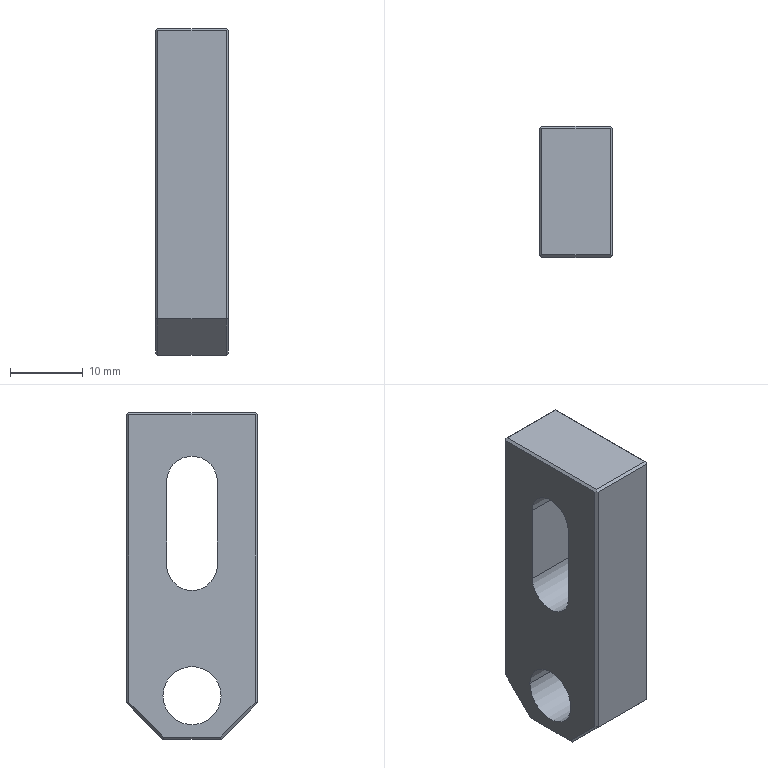Part | NX | 1 solid | 28 faces | box 10 x 18 x 45 mm | volume 6146 mm3 | plane 24 | cylinder 4 | commonest cylinder face diameters 7 x2 8 x2
STEP:
#1=CARTESIAN_POINT('',(-203.3,43.05,26.5));
#2=VERTEX_POINT('',#1);
#3=CARTESIAN_POINT('',(-212.7,43.05,26.5));
#4=VERTEX_POINT('',#3);
#5=CARTESIAN_POINT('',(-208.,43.05,26.5));
#6=DIRECTION('',(-1.,0.,0.));
#7=VECTOR('',#6,1000.);
#8=LINE('',#5,#7);
#9=EDGE_CURVE('',#2,#4,#8,.T.);
#10=ORIENTED_EDGE('',*,*,#9,.F.);
#11=CARTESIAN_POINT('',(-203.3,60.45,26.5));
#12=VERTEX_POINT('',#11);
#13=CARTESIAN_POINT('',(-203.3,51.75,26.5));
#14=DIRECTION('',(0.,1.,0.));
#15=VECTOR('',#14,1000.);
#16=LINE('',#13,#15);
#17=EDGE_CURVE('',#2,#12,#16,.T.);
#18=ORIENTED_EDGE('',*,*,#17,.T.);
#19=CARTESIAN_POINT('',(-212.7,60.45,26.5));
#20=VERTEX_POINT('',#19);
#21=CARTESIAN_POINT('',(-208.,60.45,26.5));
#22=DIRECTION('',(1.,0.,0.));
#23=VECTOR('',#22,1000.);
#24=LINE('',#21,#23);
#25=EDGE_CURVE('',#20,#12,#24,.T.);
#26=ORIENTED_EDGE('',*,*,#25,.F.);
#27=CARTESIAN_POINT('',(-212.7,51.75,26.5));
#28=DIRECTION('',(0.,1.,0.));
#29=VECTOR('',#28,1000.);
#30=LINE('',#27,#29);
#31=EDGE_CURVE('',#4,#20,#30,.T.);
#32=ORIENTED_EDGE('',*,*,#31,.F.);
#33=EDGE_LOOP('',(#10,#18,#26,#32));
#34=FACE_BOUND('',#33,.T.);
#35=CARTESIAN_POINT('',(-203.,60.75,26.5));
#36=DIRECTION('',(0.,0.,1.));
#37=DIRECTION('',(1.,0.,0.));
#38=AXIS2_PLACEMENT_3D('',#35,#36,#37);
#39=PLANE('',#38);
#40=ADVANCED_FACE('',(#34),#39,.T.);
#41=CARTESIAN_POINT('',(-203.3,60.75,-13.5));
#42=VERTEX_POINT('',#41);
#43=CARTESIAN_POINT('',(-212.7,60.75,-13.5));
#44=VERTEX_POINT('',#43);
#45=CARTESIAN_POINT('',(-208.,60.75,-13.5));
#46=DIRECTION('',(-1.,0.,0.));
#47=VECTOR('',#46,1000.);
#48=LINE('',#45,#47);
#49=EDGE_CURVE('',#42,#44,#48,.T.);
#50=ORIENTED_EDGE('',*,*,#49,.T.);
#51=CARTESIAN_POINT('',(-212.7,60.75,26.2));
#52=VERTEX_POINT('',#51);
#53=CARTESIAN_POINT('',(-212.7,60.75,6.5));
#54=DIRECTION('',(0.,0.,-1.));
#55=VECTOR('',#54,1000.);
#56=LINE('',#53,#55);
#57=EDGE_CURVE('',#52,#44,#56,.T.);
#58=ORIENTED_EDGE('',*,*,#57,.F.);
#59=CARTESIAN_POINT('',(-203.3,60.75,26.2));
#60=VERTEX_POINT('',#59);
#61=CARTESIAN_POINT('',(-208.,60.75,26.2));
#62=DIRECTION('',(1.,0.,0.));
#63=VECTOR('',#62,1000.);
#64=LINE('',#61,#63);
#65=EDGE_CURVE('',#52,#60,#64,.T.);
#66=ORIENTED_EDGE('',*,*,#65,.T.);
#67=CARTESIAN_POINT('',(-203.3,60.75,6.5));
#68=DIRECTION('',(0.,0.,-1.));
#69=VECTOR('',#68,1000.);
#70=LINE('',#67,#69);
#71=EDGE_CURVE('',#60,#42,#70,.T.);
#72=ORIENTED_EDGE('',*,*,#71,.T.);
#73=EDGE_LOOP('',(#50,#58,#66,#72));
#74=FACE_BOUND('',#73,.T.);
#75=CARTESIAN_POINT('',(-203.,60.75,0.5));
#76=DIRECTION('',(0.,1.,0.));
#77=DIRECTION('',(1.,0.,0.));
#78=AXIS2_PLACEMENT_3D('',#75,#76,#77);
#79=PLANE('',#78);
#80=ADVANCED_FACE('',(#74),#79,.T.);
#81=CARTESIAN_POINT('',(-212.7,47.75,-18.5));
#82=VERTEX_POINT('',#81);
#83=CARTESIAN_POINT('',(-203.3,47.75,-18.5));
#84=VERTEX_POINT('',#83);
#85=CARTESIAN_POINT('',(-208.,47.75,-18.5));
#86=DIRECTION('',(1.,0.,0.));
#87=VECTOR('',#86,1000.);
#88=LINE('',#85,#87);
#89=EDGE_CURVE('',#82,#84,#88,.T.);
#90=ORIENTED_EDGE('',*,*,#89,.F.);
#91=CARTESIAN_POINT('',(-212.7,55.75,-18.5));
#92=VERTEX_POINT('',#91);
#93=CARTESIAN_POINT('',(-212.7,51.75,-18.5));
#94=DIRECTION('',(0.,-1.,0.));
#95=VECTOR('',#94,1000.);
#96=LINE('',#93,#95);
#97=EDGE_CURVE('',#92,#82,#96,.T.);
#98=ORIENTED_EDGE('',*,*,#97,.F.);
#99=CARTESIAN_POINT('',(-203.3,55.75,-18.5));
#100=VERTEX_POINT('',#99);
#101=CARTESIAN_POINT('',(-208.,55.75,-18.5));
#102=DIRECTION('',(-1.,0.,0.));
#103=VECTOR('',#102,1000.);
#104=LINE('',#101,#103);
#105=EDGE_CURVE('',#100,#92,#104,.T.);
#106=ORIENTED_EDGE('',*,*,#105,.F.);
#107=CARTESIAN_POINT('',(-203.3,51.75,-18.5));
#108=DIRECTION('',(0.,-1.,0.));
#109=VECTOR('',#108,1000.);
#110=LINE('',#107,#109);
#111=EDGE_CURVE('',#100,#84,#110,.T.);
#112=ORIENTED_EDGE('',*,*,#111,.T.);
#113=EDGE_LOOP('',(#90,#98,#106,#112));
#114=FACE_BOUND('',#113,.T.);
#115=CARTESIAN_POINT('',(-203.,42.75,-18.5));
#116=DIRECTION('',(0.,0.,-1.));
#117=DIRECTION('',(0.,-1.,0.));
#118=AXIS2_PLACEMENT_3D('',#115,#116,#117);
#119=PLANE('',#118);
#120=ADVANCED_FACE('',(#114),#119,.T.);
#121=CARTESIAN_POINT('',(-203.3,42.75,-13.5));
#122=VERTEX_POINT('',#121);
#123=CARTESIAN_POINT('',(-203.3,42.75,26.2));
#124=VERTEX_POINT('',#123);
#125=CARTESIAN_POINT('',(-203.3,42.75,6.5));
#126=DIRECTION('',(0.,0.,1.));
#127=VECTOR('',#126,1000.);
#128=LINE('',#125,#127);
#129=EDGE_CURVE('',#122,#124,#128,.T.);
#130=ORIENTED_EDGE('',*,*,#129,.T.);
#131=CARTESIAN_POINT('',(-212.7,42.75,26.2));
#132=VERTEX_POINT('',#131);
#133=CARTESIAN_POINT('',(-208.,42.75,26.2));
#134=DIRECTION('',(-1.,0.,0.));
#135=VECTOR('',#134,1000.);
#136=LINE('',#133,#135);
#137=EDGE_CURVE('',#124,#132,#136,.T.);
#138=ORIENTED_EDGE('',*,*,#137,.T.);
#139=CARTESIAN_POINT('',(-212.7,42.75,-13.5));
#140=VERTEX_POINT('',#139);
#141=CARTESIAN_POINT('',(-212.7,42.75,6.5));
#142=DIRECTION('',(0.,0.,1.));
#143=VECTOR('',#142,1000.);
#144=LINE('',#141,#143);
#145=EDGE_CURVE('',#140,#132,#144,.T.);
#146=ORIENTED_EDGE('',*,*,#145,.F.);
#147=CARTESIAN_POINT('',(-208.,42.75,-13.5));
#148=DIRECTION('',(1.,0.,0.));
#149=VECTOR('',#148,1000.);
#150=LINE('',#147,#149);
#151=EDGE_CURVE('',#140,#122,#150,.T.);
#152=ORIENTED_EDGE('',*,*,#151,.T.);
#153=EDGE_LOOP('',(#130,#138,#146,#152));
#154=FACE_BOUND('',#153,.T.);
#155=CARTESIAN_POINT('',(-203.,42.75,18.5));
#156=DIRECTION('',(0.,-1.,0.));
#157=DIRECTION('',(0.,0.,-1.));
#158=AXIS2_PLACEMENT_3D('',#155,#156,#157);
#159=PLANE('',#158);
#160=ADVANCED_FACE('',(#154),#159,.T.);
#161=CARTESIAN_POINT('',(-203.,55.75,-12.5));
#162=VERTEX_POINT('',#161);
#163=CARTESIAN_POINT('',(-203.,47.75,-12.5));
#164=VERTEX_POINT('',#163);
#165=CARTESIAN_POINT('',(-203.,51.75,-12.5));
#166=DIRECTION('',(-1.,0.,0.));
#167=DIRECTION('',(0.,-1.,0.));
#168=AXIS2_PLACEMENT_3D('',#165,#166,#167);
#169=CIRCLE('',#168,4.);
#170=EDGE_CURVE('',#162,#164,#169,.T.);
#171=ORIENTED_EDGE('',*,*,#170,.F.);
#172=CARTESIAN_POINT('',(-213.,55.75,-12.5));
#173=VERTEX_POINT('',#172);
#174=CARTESIAN_POINT('',(-202.,55.75,-12.5));
#175=DIRECTION('',(-1.,0.,0.));
#176=VECTOR('',#175,1000.);
#177=LINE('',#174,#176);
#178=EDGE_CURVE('',#173,#162,#177,.F.);
#179=ORIENTED_EDGE('',*,*,#178,.F.);
#180=CARTESIAN_POINT('',(-213.,47.75,-12.5));
#181=VERTEX_POINT('',#180);
#182=CARTESIAN_POINT('',(-213.,51.75,-12.5));
#183=DIRECTION('',(-1.,0.,0.));
#184=DIRECTION('',(0.,-1.,0.));
#185=AXIS2_PLACEMENT_3D('',#182,#183,#184);
#186=CIRCLE('',#185,4.);
#187=EDGE_CURVE('',#173,#181,#186,.T.);
#188=ORIENTED_EDGE('',*,*,#187,.T.);
#189=CARTESIAN_POINT('',(-202.,47.75,-12.5));
#190=DIRECTION('',(-1.,0.,0.));
#191=VECTOR('',#190,1000.);
#192=LINE('',#189,#191);
#193=EDGE_CURVE('',#181,#164,#192,.F.);
#194=ORIENTED_EDGE('',*,*,#193,.T.);
#195=EDGE_LOOP('',(#171,#179,#188,#194));
#196=FACE_BOUND('',#195,.T.);
#197=CARTESIAN_POINT('',(-202.,51.75,-12.5));
#198=DIRECTION('',(-1.,0.,0.));
#199=DIRECTION('',(0.,-1.,0.));
#200=AXIS2_PLACEMENT_3D('',#197,#198,#199);
#201=CYLINDRICAL_SURFACE('',#200,4.);
#202=ADVANCED_FACE('',(#196),#201,.F.);
#203=CARTESIAN_POINT('',(-203.3,58.25,-16.));
#204=DIRECTION('',(0.,0.7071,0.7071));
#205=VECTOR('',#204,1000.);
#206=LINE('',#203,#205);
#207=EDGE_CURVE('',#100,#42,#206,.T.);
#208=ORIENTED_EDGE('',*,*,#207,.F.);
#209=ORIENTED_EDGE('',*,*,#105,.T.);
#210=CARTESIAN_POINT('',(-212.7,58.25,-16.));
#211=DIRECTION('',(0.,0.7071,0.7071));
#212=VECTOR('',#211,1000.);
#213=LINE('',#210,#212);
#214=EDGE_CURVE('',#92,#44,#213,.T.);
#215=ORIENTED_EDGE('',*,*,#214,.T.);
#216=ORIENTED_EDGE('',*,*,#49,.F.);
#217=EDGE_LOOP('',(#208,#209,#215,#216));
#218=FACE_BOUND('',#217,.T.);
#219=CARTESIAN_POINT('',(-208.,58.25,-16.));
#220=DIRECTION('',(0.,0.7071,-0.7071));
#221=DIRECTION('',(-1.,0.,0.));
#222=AXIS2_PLACEMENT_3D('',#219,#220,#221);
#223=PLANE('',#222);
#224=ADVANCED_FACE('',(#218),#223,.T.);
#225=CARTESIAN_POINT('',(-203.3,45.25,-16.));
#226=DIRECTION('',(0.,-0.7071,0.7071));
#227=VECTOR('',#226,1000.);
#228=LINE('',#225,#227);
#229=EDGE_CURVE('',#84,#122,#228,.T.);
#230=ORIENTED_EDGE('',*,*,#229,.T.);
#231=ORIENTED_EDGE('',*,*,#151,.F.);
#232=CARTESIAN_POINT('',(-212.7,45.25,-16.));
#233=DIRECTION('',(0.,-0.7071,0.7071));
#234=VECTOR('',#233,1000.);
#235=LINE('',#232,#234);
#236=EDGE_CURVE('',#82,#140,#235,.T.);
#237=ORIENTED_EDGE('',*,*,#236,.F.);
#238=ORIENTED_EDGE('',*,*,#89,.T.);
#239=EDGE_LOOP('',(#230,#231,#237,#238));
#240=FACE_BOUND('',#239,.T.);
#241=CARTESIAN_POINT('',(-208.,45.25,-16.));
#242=DIRECTION('',(0.,0.7071,0.7071));
#243=DIRECTION('',(1.,0.,0.));
#244=AXIS2_PLACEMENT_3D('',#241,#242,#243);
#245=PLANE('',#244);
#246=ADVANCED_FACE('',(#240),#245,.F.);
#247=ORIENTED_EDGE('',*,*,#25,.T.);
#248=CARTESIAN_POINT('',(-203.15,60.6,26.35));
#249=VERTEX_POINT('',#248);
#250=CARTESIAN_POINT('',(-186.932,76.818,10.132));
#251=DIRECTION('',(0.5774,0.5774,-0.5774));
#252=VECTOR('',#251,1000.);
#253=LINE('',#250,#252);
#254=EDGE_CURVE('',#12,#249,#253,.T.);
#255=ORIENTED_EDGE('',*,*,#254,.T.);
#256=CARTESIAN_POINT('',(-219.368,76.818,10.132));
#257=DIRECTION('',(-0.5774,0.5774,-0.5774));
#258=VECTOR('',#257,1000.);
#259=LINE('',#256,#258);
#260=EDGE_CURVE('',#249,#60,#259,.T.);
#261=ORIENTED_EDGE('',*,*,#260,.T.);
#262=ORIENTED_EDGE('',*,*,#65,.F.);
#263=CARTESIAN_POINT('',(-212.85,60.6,26.35));
#264=VERTEX_POINT('',#263);
#265=CARTESIAN_POINT('',(-203.,70.45,16.5));
#266=DIRECTION('',(-0.5774,-0.5774,0.5774));
#267=VECTOR('',#266,1000.);
#268=LINE('',#265,#267);
#269=EDGE_CURVE('',#52,#264,#268,.T.);
#270=ORIENTED_EDGE('',*,*,#269,.T.);
#271=CARTESIAN_POINT('',(-203.,50.75,36.2));
#272=DIRECTION('',(0.5774,-0.5774,0.5774));
#273=VECTOR('',#272,1000.);
#274=LINE('',#271,#273);
#275=EDGE_CURVE('',#264,#20,#274,.T.);
#276=ORIENTED_EDGE('',*,*,#275,.T.);
#277=EDGE_LOOP('',(#247,#255,#261,#262,#270,#276));
#278=FACE_BOUND('',#277,.T.);
#279=CARTESIAN_POINT('',(-208.,60.6,26.35));
#280=DIRECTION('',(0.,-0.7071,-0.7071));
#281=DIRECTION('',(0.,0.7071,-0.7071));
#282=AXIS2_PLACEMENT_3D('',#279,#280,#281);
#283=PLANE('',#282);
#284=ADVANCED_FACE('',(#278),#283,.F.);
#285=ORIENTED_EDGE('',*,*,#9,.T.);
#286=CARTESIAN_POINT('',(-212.85,42.9,26.35));
#287=VERTEX_POINT('',#286);
#288=CARTESIAN_POINT('',(-203.,52.75,36.2));
#289=DIRECTION('',(-0.5774,-0.5774,-0.5774));
#290=VECTOR('',#289,1000.);
#291=LINE('',#288,#290);
#292=EDGE_CURVE('',#4,#287,#291,.T.);
#293=ORIENTED_EDGE('',*,*,#292,.T.);
#294=CARTESIAN_POINT('',(-203.,33.05,16.5));
#295=DIRECTION('',(-0.5774,0.5774,0.5774));
#296=VECTOR('',#295,1000.);
#297=LINE('',#294,#296);
#298=EDGE_CURVE('',#132,#287,#297,.T.);
#299=ORIENTED_EDGE('',*,*,#298,.F.);
#300=ORIENTED_EDGE('',*,*,#137,.F.);
#301=CARTESIAN_POINT('',(-203.15,42.9,26.35));
#302=VERTEX_POINT('',#301);
#303=CARTESIAN_POINT('',(-219.368,26.682,10.132));
#304=DIRECTION('',(0.5774,0.5774,0.5774));
#305=VECTOR('',#304,1000.);
#306=LINE('',#303,#305);
#307=EDGE_CURVE('',#124,#302,#306,.T.);
#308=ORIENTED_EDGE('',*,*,#307,.T.);
#309=CARTESIAN_POINT('',(-186.932,26.682,10.132));
#310=DIRECTION('',(0.5774,-0.5774,-0.5774));
#311=VECTOR('',#310,1000.);
#312=LINE('',#309,#311);
#313=EDGE_CURVE('',#2,#302,#312,.T.);
#314=ORIENTED_EDGE('',*,*,#313,.F.);
#315=EDGE_LOOP('',(#285,#293,#299,#300,#308,#314));
#316=FACE_BOUND('',#315,.T.);
#317=CARTESIAN_POINT('',(-208.,42.9,26.35));
#318=DIRECTION('',(0.,0.7071,-0.7071));
#319=DIRECTION('',(-1.,0.,0.));
#320=AXIS2_PLACEMENT_3D('',#317,#318,#319);
#321=PLANE('',#320);
#322=ADVANCED_FACE('',(#316),#321,.F.);
#323=ORIENTED_EDGE('',*,*,#236,.T.);
#324=CARTESIAN_POINT('',(-213.,43.05,-13.376));
#325=VERTEX_POINT('',#324);
#326=CARTESIAN_POINT('',(-203.,33.05,-17.518));
#327=DIRECTION('',(-0.6786,0.6786,0.2811));
#328=VECTOR('',#327,1000.);
#329=LINE('',#326,#328);
#330=EDGE_CURVE('',#140,#325,#329,.T.);
#331=ORIENTED_EDGE('',*,*,#330,.T.);
#332=CARTESIAN_POINT('',(-213.,47.874,-18.2));
#333=VERTEX_POINT('',#332);
#334=CARTESIAN_POINT('',(-213.,45.462,-15.788));
#335=DIRECTION('',(0.,-0.7071,0.7071));
#336=VECTOR('',#335,1000.);
#337=LINE('',#334,#336);
#338=EDGE_CURVE('',#333,#325,#337,.T.);
#339=ORIENTED_EDGE('',*,*,#338,.F.);
#340=CARTESIAN_POINT('',(-203.,43.732,-28.2));
#341=DIRECTION('',(-0.6786,0.2811,0.6786));
#342=VECTOR('',#341,1000.);
#343=LINE('',#340,#342);
#344=EDGE_CURVE('',#82,#333,#343,.T.);
#345=ORIENTED_EDGE('',*,*,#344,.F.);
#346=EDGE_LOOP('',(#323,#331,#339,#345));
#347=FACE_BOUND('',#346,.T.);
#348=CARTESIAN_POINT('',(-212.85,45.356,-15.894));
#349=DIRECTION('',(0.7071,0.5,0.5));
#350=DIRECTION('',(0.,0.7071,-0.7071));
#351=AXIS2_PLACEMENT_3D('',#348,#349,#350);
#352=PLANE('',#351);
#353=ADVANCED_FACE('',(#347),#352,.F.);
#354=ORIENTED_EDGE('',*,*,#214,.F.);
#355=CARTESIAN_POINT('',(-213.,55.626,-18.2));
#356=VERTEX_POINT('',#355);
#357=CARTESIAN_POINT('',(-241.332,43.89,10.132));
#358=DIRECTION('',(0.6786,0.2811,-0.6786));
#359=VECTOR('',#358,1000.);
#360=LINE('',#357,#359);
#361=EDGE_CURVE('',#356,#92,#360,.T.);
#362=ORIENTED_EDGE('',*,*,#361,.F.);
#363=CARTESIAN_POINT('',(-213.,60.45,-13.376));
#364=VERTEX_POINT('',#363);
#365=CARTESIAN_POINT('',(-213.,58.038,-15.788));
#366=DIRECTION('',(0.,0.7071,0.7071));
#367=VECTOR('',#366,1000.);
#368=LINE('',#365,#367);
#369=EDGE_CURVE('',#356,#364,#368,.T.);
#370=ORIENTED_EDGE('',*,*,#369,.T.);
#371=CARTESIAN_POINT('',(-203.,70.45,-17.518));
#372=DIRECTION('',(-0.6786,-0.6786,0.2811));
#373=VECTOR('',#372,1000.);
#374=LINE('',#371,#373);
#375=EDGE_CURVE('',#44,#364,#374,.T.);
#376=ORIENTED_EDGE('',*,*,#375,.F.);
#377=EDGE_LOOP('',(#354,#362,#370,#376));
#378=FACE_BOUND('',#377,.T.);
#379=CARTESIAN_POINT('',(-212.85,58.144,-15.894));
#380=DIRECTION('',(-0.7071,0.5,-0.5));
#381=DIRECTION('',(-0.5774,0.,0.8165));
#382=AXIS2_PLACEMENT_3D('',#379,#380,#381);
#383=PLANE('',#382);
#384=ADVANCED_FACE('',(#378),#383,.T.);
#385=ORIENTED_EDGE('',*,*,#207,.T.);
#386=CARTESIAN_POINT('',(-203.,60.45,-13.376));
#387=VERTEX_POINT('',#386);
#388=CARTESIAN_POINT('',(-203.,60.45,-13.376));
#389=DIRECTION('',(0.6786,-0.6786,0.2811));
#390=VECTOR('',#389,1000.);
#391=LINE('',#388,#390);
#392=EDGE_CURVE('',#42,#387,#391,.T.);
#393=ORIENTED_EDGE('',*,*,#392,.T.);
#394=CARTESIAN_POINT('',(-203.,55.626,-18.2));
#395=VERTEX_POINT('',#394);
#396=CARTESIAN_POINT('',(-203.,58.038,-15.788));
#397=DIRECTION('',(0.,0.7071,0.7071));
#398=VECTOR('',#397,1000.);
#399=LINE('',#396,#398);
#400=EDGE_CURVE('',#395,#387,#399,.T.);
#401=ORIENTED_EDGE('',*,*,#400,.F.);
#402=CARTESIAN_POINT('',(-174.668,43.89,10.132));
#403=DIRECTION('',(-0.6786,0.2811,-0.6786));
#404=VECTOR('',#403,1000.);
#405=LINE('',#402,#404);
#406=EDGE_CURVE('',#395,#100,#405,.T.);
#407=ORIENTED_EDGE('',*,*,#406,.T.);
#408=EDGE_LOOP('',(#385,#393,#401,#407));
#409=FACE_BOUND('',#408,.T.);
#410=CARTESIAN_POINT('',(-203.15,58.144,-15.894));
#411=DIRECTION('',(-0.7071,-0.5,0.5));
#412=DIRECTION('',(-0.5774,0.8165,0.));
#413=AXIS2_PLACEMENT_3D('',#410,#411,#412);
#414=PLANE('',#413);
#415=ADVANCED_FACE('',(#409),#414,.F.);
#416=ORIENTED_EDGE('',*,*,#229,.F.);
#417=CARTESIAN_POINT('',(-203.,47.874,-18.2));
#418=VERTEX_POINT('',#417);
#419=CARTESIAN_POINT('',(-174.668,59.61,10.132));
#420=DIRECTION('',(0.6786,0.2811,0.6786));
#421=VECTOR('',#420,1000.);
#422=LINE('',#419,#421);
#423=EDGE_CURVE('',#84,#418,#422,.T.);
#424=ORIENTED_EDGE('',*,*,#423,.T.);
#425=CARTESIAN_POINT('',(-203.,43.05,-13.376));
#426=VERTEX_POINT('',#425);
#427=CARTESIAN_POINT('',(-203.,45.462,-15.788));
#428=DIRECTION('',(0.,-0.7071,0.7071));
#429=VECTOR('',#428,1000.);
#430=LINE('',#427,#429);
#431=EDGE_CURVE('',#418,#426,#430,.T.);
#432=ORIENTED_EDGE('',*,*,#431,.T.);
#433=CARTESIAN_POINT('',(-192.115,53.935,-8.867));
#434=DIRECTION('',(-0.6786,-0.6786,-0.2811));
#435=VECTOR('',#434,1000.);
#436=LINE('',#433,#435);
#437=EDGE_CURVE('',#426,#122,#436,.T.);
#438=ORIENTED_EDGE('',*,*,#437,.T.);
#439=EDGE_LOOP('',(#416,#424,#432,#438));
#440=FACE_BOUND('',#439,.T.);
#441=CARTESIAN_POINT('',(-203.15,45.356,-15.894));
#442=DIRECTION('',(0.7071,-0.5,-0.5));
#443=DIRECTION('',(0.,-0.7071,0.7071));
#444=AXIS2_PLACEMENT_3D('',#441,#442,#443);
#445=PLANE('',#444);
#446=ADVANCED_FACE('',(#440),#445,.T.);
#447=ORIENTED_EDGE('',*,*,#193,.F.);
#448=CARTESIAN_POINT('',(-213.,51.75,-12.5));
#449=DIRECTION('',(-1.,0.,0.));
#450=DIRECTION('',(0.,-1.,0.));
#451=AXIS2_PLACEMENT_3D('',#448,#449,#450);
#452=CIRCLE('',#451,4.);
#453=EDGE_CURVE('',#181,#173,#452,.T.);
#454=ORIENTED_EDGE('',*,*,#453,.T.);
#455=ORIENTED_EDGE('',*,*,#178,.T.);
#456=CARTESIAN_POINT('',(-203.,51.75,-12.5));
#457=DIRECTION('',(-1.,0.,0.));
#458=DIRECTION('',(0.,-1.,0.));
#459=AXIS2_PLACEMENT_3D('',#456,#457,#458);
#460=CIRCLE('',#459,4.);
#461=EDGE_CURVE('',#164,#162,#460,.T.);
#462=ORIENTED_EDGE('',*,*,#461,.F.);
#463=EDGE_LOOP('',(#447,#454,#455,#462));
#464=FACE_BOUND('',#463,.T.);
#465=CARTESIAN_POINT('',(-202.,51.75,-12.5));
#466=DIRECTION('',(-1.,0.,0.));
#467=DIRECTION('',(0.,-1.,0.));
#468=AXIS2_PLACEMENT_3D('',#465,#466,#467);
#469=CYLINDRICAL_SURFACE('',#468,4.);
#470=ADVANCED_FACE('',(#464),#469,.F.);
#471=CARTESIAN_POINT('',(-213.,51.75,-18.2));
#472=DIRECTION('',(0.,-1.,0.));
#473=VECTOR('',#472,1000.);
#474=LINE('',#471,#473);
#475=EDGE_CURVE('',#356,#333,#474,.T.);
#476=ORIENTED_EDGE('',*,*,#475,.T.);
#477=ORIENTED_EDGE('',*,*,#338,.T.);
#478=CARTESIAN_POINT('',(-213.,43.05,26.2));
#479=VERTEX_POINT('',#478);
#480=CARTESIAN_POINT('',(-213.,43.05,6.5));
#481=DIRECTION('',(0.,0.,1.));
#482=VECTOR('',#481,1000.);
#483=LINE('',#480,#482);
#484=EDGE_CURVE('',#325,#479,#483,.T.);
#485=ORIENTED_EDGE('',*,*,#484,.T.);
#486=CARTESIAN_POINT('',(-213.,60.45,26.2));
#487=VERTEX_POINT('',#486);
#488=CARTESIAN_POINT('',(-213.,51.75,26.2));
#489=DIRECTION('',(0.,1.,0.));
#490=VECTOR('',#489,1000.);
#491=LINE('',#488,#490);
#492=EDGE_CURVE('',#479,#487,#491,.T.);
#493=ORIENTED_EDGE('',*,*,#492,.T.);
#494=CARTESIAN_POINT('',(-213.,60.45,6.5));
#495=DIRECTION('',(0.,0.,-1.));
#496=VECTOR('',#495,1000.);
#497=LINE('',#494,#496);
#498=EDGE_CURVE('',#487,#364,#497,.T.);
#499=ORIENTED_EDGE('',*,*,#498,.T.);
#500=ORIENTED_EDGE('',*,*,#369,.F.);
#501=EDGE_LOOP('',(#476,#477,#485,#493,#499,#500));
#502=FACE_BOUND('',#501,.T.);
#503=ORIENTED_EDGE('',*,*,#187,.F.);
#504=ORIENTED_EDGE('',*,*,#453,.F.);
#505=EDGE_LOOP('',(#503,#504));
#506=FACE_BOUND('',#505,.T.);
#507=CARTESIAN_POINT('',(-213.,48.25,5.5));
#508=VERTEX_POINT('',#507);
#509=CARTESIAN_POINT('',(-213.,48.25,17.));
#510=VERTEX_POINT('',#509);
#511=CARTESIAN_POINT('',(-213.,48.25,10.132));
#512=DIRECTION('',(0.,0.,1.));
#513=VECTOR('',#512,1000.);
#514=LINE('',#511,#513);
#515=EDGE_CURVE('',#508,#510,#514,.T.);
#516=ORIENTED_EDGE('',*,*,#515,.F.);
#517=CARTESIAN_POINT('',(-213.,55.25,5.5));
#518=VERTEX_POINT('',#517);
#519=CARTESIAN_POINT('',(-213.,51.75,5.5));
#520=DIRECTION('',(-1.,0.,0.));
#521=DIRECTION('',(0.,-1.,0.));
#522=AXIS2_PLACEMENT_3D('',#519,#520,#521);
#523=CIRCLE('',#522,3.5);
#524=EDGE_CURVE('',#518,#508,#523,.T.);
#525=ORIENTED_EDGE('',*,*,#524,.F.);
#526=CARTESIAN_POINT('',(-213.,55.25,17.));
#527=VERTEX_POINT('',#526);
#528=CARTESIAN_POINT('',(-213.,55.25,10.132));
#529=DIRECTION('',(0.,0.,-1.));
#530=VECTOR('',#529,1000.);
#531=LINE('',#528,#530);
#532=EDGE_CURVE('',#527,#518,#531,.T.);
#533=ORIENTED_EDGE('',*,*,#532,.F.);
#534=CARTESIAN_POINT('',(-213.,51.75,17.));
#535=DIRECTION('',(-1.,0.,0.));
#536=DIRECTION('',(0.,-1.,0.));
#537=AXIS2_PLACEMENT_3D('',#534,#535,#536);
#538=CIRCLE('',#537,3.5);
#539=EDGE_CURVE('',#510,#527,#538,.T.);
#540=ORIENTED_EDGE('',*,*,#539,.F.);
#541=EDGE_LOOP('',(#516,#525,#533,#540));
#542=FACE_BOUND('',#541,.T.);
#543=CARTESIAN_POINT('',(-213.,53.935,10.132));
#544=DIRECTION('',(-1.,0.,0.));
#545=DIRECTION('',(0.,0.,1.));
#546=AXIS2_PLACEMENT_3D('',#543,#544,#545);
#547=PLANE('',#546);
#548=ADVANCED_FACE('',(#502,#506,#542),#547,.T.);
#549=ORIENTED_EDGE('',*,*,#475,.F.);
#550=ORIENTED_EDGE('',*,*,#361,.T.);
#551=ORIENTED_EDGE('',*,*,#97,.T.);
#552=ORIENTED_EDGE('',*,*,#344,.T.);
#553=EDGE_LOOP('',(#549,#550,#551,#552));
#554=FACE_BOUND('',#553,.T.);
#555=CARTESIAN_POINT('',(-212.85,51.75,-18.35));
#556=DIRECTION('',(-0.7071,0.,-0.7071));
#557=DIRECTION('',(-0.7071,0.,0.7071));
#558=AXIS2_PLACEMENT_3D('',#555,#556,#557);
#559=PLANE('',#558);
#560=ADVANCED_FACE('',(#554),#559,.T.);
#561=CARTESIAN_POINT('',(-203.,55.25,17.));
#562=VERTEX_POINT('',#561);
#563=CARTESIAN_POINT('',(-203.,55.25,5.5));
#564=VERTEX_POINT('',#563);
#565=CARTESIAN_POINT('',(-203.,55.25,10.132));
#566=DIRECTION('',(0.,0.,-1.));
#567=VECTOR('',#566,1000.);
#568=LINE('',#565,#567);
#569=EDGE_CURVE('',#562,#564,#568,.T.);
#570=ORIENTED_EDGE('',*,*,#569,.F.);
#571=CARTESIAN_POINT('',(-202.,55.25,17.));
#572=DIRECTION('',(-1.,0.,0.));
#573=VECTOR('',#572,1000.);
#574=LINE('',#571,#573);
#575=EDGE_CURVE('',#562,#527,#574,.T.);
#576=ORIENTED_EDGE('',*,*,#575,.T.);
#577=ORIENTED_EDGE('',*,*,#532,.T.);
#578=CARTESIAN_POINT('',(-202.,55.25,5.5));
#579=DIRECTION('',(-1.,0.,0.));
#580=VECTOR('',#579,1000.);
#581=LINE('',#578,#580);
#582=EDGE_CURVE('',#564,#518,#581,.T.);
#583=ORIENTED_EDGE('',*,*,#582,.F.);
#584=EDGE_LOOP('',(#570,#576,#577,#583));
#585=FACE_BOUND('',#584,.T.);
#586=CARTESIAN_POINT('',(-202.,55.25,5.5));
#587=DIRECTION('',(0.,1.,0.));
#588=DIRECTION('',(1.,0.,0.));
#589=AXIS2_PLACEMENT_3D('',#586,#587,#588);
#590=PLANE('',#589);
#591=ADVANCED_FACE('',(#585),#590,.F.);
#592=CARTESIAN_POINT('',(-203.,48.25,5.5));
#593=VERTEX_POINT('',#592);
#594=CARTESIAN_POINT('',(-203.,51.75,5.5));
#595=DIRECTION('',(-1.,0.,0.));
#596=DIRECTION('',(0.,-1.,0.));
#597=AXIS2_PLACEMENT_3D('',#594,#595,#596);
#598=CIRCLE('',#597,3.5);
#599=EDGE_CURVE('',#564,#593,#598,.T.);
#600=ORIENTED_EDGE('',*,*,#599,.F.);
#601=ORIENTED_EDGE('',*,*,#582,.T.);
#602=ORIENTED_EDGE('',*,*,#524,.T.);
#603=CARTESIAN_POINT('',(-202.,48.25,5.5));
#604=DIRECTION('',(-1.,0.,0.));
#605=VECTOR('',#604,1000.);
#606=LINE('',#603,#605);
#607=EDGE_CURVE('',#593,#508,#606,.T.);
#608=ORIENTED_EDGE('',*,*,#607,.F.);
#609=EDGE_LOOP('',(#600,#601,#602,#608));
#610=FACE_BOUND('',#609,.T.);
#611=CARTESIAN_POINT('',(-202.,51.75,5.5));
#612=DIRECTION('',(-1.,0.,0.));
#613=DIRECTION('',(0.,-1.,0.));
#614=AXIS2_PLACEMENT_3D('',#611,#612,#613);
#615=CYLINDRICAL_SURFACE('',#614,3.5);
#616=ADVANCED_FACE('',(#610),#615,.F.);
#617=ORIENTED_EDGE('',*,*,#539,.T.);
#618=ORIENTED_EDGE('',*,*,#575,.F.);
#619=CARTESIAN_POINT('',(-203.,48.25,17.));
#620=VERTEX_POINT('',#619);
#621=CARTESIAN_POINT('',(-203.,51.75,17.));
#622=DIRECTION('',(-1.,0.,0.));
#623=DIRECTION('',(0.,-1.,0.));
#624=AXIS2_PLACEMENT_3D('',#621,#622,#623);
#625=CIRCLE('',#624,3.5);
#626=EDGE_CURVE('',#620,#562,#625,.T.);
#627=ORIENTED_EDGE('',*,*,#626,.F.);
#628=CARTESIAN_POINT('',(-202.,48.25,17.));
#629=DIRECTION('',(-1.,0.,0.));
#630=VECTOR('',#629,1000.);
#631=LINE('',#628,#630);
#632=EDGE_CURVE('',#620,#510,#631,.T.);
#633=ORIENTED_EDGE('',*,*,#632,.T.);
#634=EDGE_LOOP('',(#617,#618,#627,#633));
#635=FACE_BOUND('',#634,.T.);
#636=CARTESIAN_POINT('',(-202.,51.75,17.));
#637=DIRECTION('',(-1.,0.,0.));
#638=DIRECTION('',(0.,-1.,0.));
#639=AXIS2_PLACEMENT_3D('',#636,#637,#638);
#640=CYLINDRICAL_SURFACE('',#639,3.5);
#641=ADVANCED_FACE('',(#635),#640,.F.);
#642=ORIENTED_EDGE('',*,*,#498,.F.);
#643=CARTESIAN_POINT('',(-203.,70.45,36.2));
#644=DIRECTION('',(0.5774,0.5774,0.5774));
#645=VECTOR('',#644,1000.);
#646=LINE('',#643,#645);
#647=EDGE_CURVE('',#487,#264,#646,.T.);
#648=ORIENTED_EDGE('',*,*,#647,.T.);
#649=ORIENTED_EDGE('',*,*,#269,.F.);
#650=ORIENTED_EDGE('',*,*,#57,.T.);
#651=ORIENTED_EDGE('',*,*,#375,.T.);
#652=EDGE_LOOP('',(#642,#648,#649,#650,#651));
#653=FACE_BOUND('',#652,.T.);
#654=CARTESIAN_POINT('',(-212.85,60.6,6.5));
#655=DIRECTION('',(-0.7071,0.7071,0.));
#656=DIRECTION('',(0.,0.,1.));
#657=AXIS2_PLACEMENT_3D('',#654,#655,#656);
#658=PLANE('',#657);
#659=ADVANCED_FACE('',(#653),#658,.T.);
#660=ORIENTED_EDGE('',*,*,#492,.F.);
#661=CARTESIAN_POINT('',(-203.,33.05,36.2));
#662=DIRECTION('',(0.5774,-0.5774,0.5774));
#663=VECTOR('',#662,1000.);
#664=LINE('',#661,#663);
#665=EDGE_CURVE('',#479,#287,#664,.T.);
#666=ORIENTED_EDGE('',*,*,#665,.T.);
#667=ORIENTED_EDGE('',*,*,#292,.F.);
#668=ORIENTED_EDGE('',*,*,#31,.T.);
#669=ORIENTED_EDGE('',*,*,#275,.F.);
#670=ORIENTED_EDGE('',*,*,#647,.F.);
#671=EDGE_LOOP('',(#660,#666,#667,#668,#669,#670));
#672=FACE_BOUND('',#671,.T.);
#673=CARTESIAN_POINT('',(-212.85,51.75,26.35));
#674=DIRECTION('',(-0.7071,0.,0.7071));
#675=DIRECTION('',(0.,1.,0.));
#676=AXIS2_PLACEMENT_3D('',#673,#674,#675);
#677=PLANE('',#676);
#678=ADVANCED_FACE('',(#672),#677,.T.);
#679=ORIENTED_EDGE('',*,*,#484,.F.);
#680=ORIENTED_EDGE('',*,*,#330,.F.);
#681=ORIENTED_EDGE('',*,*,#145,.T.);
#682=ORIENTED_EDGE('',*,*,#298,.T.);
#683=ORIENTED_EDGE('',*,*,#665,.F.);
#684=EDGE_LOOP('',(#679,#680,#681,#682,#683));
#685=FACE_BOUND('',#684,.T.);
#686=CARTESIAN_POINT('',(-212.85,42.9,6.5));
#687=DIRECTION('',(-0.7071,-0.7071,0.));
#688=DIRECTION('',(-0.7071,0.7071,0.));
#689=AXIS2_PLACEMENT_3D('',#686,#687,#688);
#690=PLANE('',#689);
#691=ADVANCED_FACE('',(#685),#690,.T.);
#692=ORIENTED_EDGE('',*,*,#515,.T.);
#693=ORIENTED_EDGE('',*,*,#632,.F.);
#694=CARTESIAN_POINT('',(-203.,48.25,10.132));
#695=DIRECTION('',(0.,0.,1.));
#696=VECTOR('',#695,1000.);
#697=LINE('',#694,#696);
#698=EDGE_CURVE('',#593,#620,#697,.T.);
#699=ORIENTED_EDGE('',*,*,#698,.F.);
#700=ORIENTED_EDGE('',*,*,#607,.T.);
#701=EDGE_LOOP('',(#692,#693,#699,#700));
#702=FACE_BOUND('',#701,.T.);
#703=CARTESIAN_POINT('',(-202.,48.25,17.));
#704=DIRECTION('',(0.,-1.,0.));
#705=DIRECTION('',(0.,0.,-1.));
#706=AXIS2_PLACEMENT_3D('',#703,#704,#705);
#707=PLANE('',#706);
#708=ADVANCED_FACE('',(#702),#707,.F.);
#709=CARTESIAN_POINT('',(-203.,60.45,26.2));
#710=VERTEX_POINT('',#709);
#711=CARTESIAN_POINT('',(-203.,60.45,6.5));
#712=DIRECTION('',(0.,0.,-1.));
#713=VECTOR('',#712,1000.);
#714=LINE('',#711,#713);
#715=EDGE_CURVE('',#710,#387,#714,.T.);
#716=ORIENTED_EDGE('',*,*,#715,.F.);
#717=CARTESIAN_POINT('',(-203.,43.05,26.2));
#718=VERTEX_POINT('',#717);
#719=CARTESIAN_POINT('',(-203.,51.75,26.2));
#720=DIRECTION('',(0.,1.,0.));
#721=VECTOR('',#720,1000.);
#722=LINE('',#719,#721);
#723=EDGE_CURVE('',#718,#710,#722,.T.);
#724=ORIENTED_EDGE('',*,*,#723,.F.);
#725=CARTESIAN_POINT('',(-203.,43.05,6.5));
#726=DIRECTION('',(0.,0.,1.));
#727=VECTOR('',#726,1000.);
#728=LINE('',#725,#727);
#729=EDGE_CURVE('',#426,#718,#728,.T.);
#730=ORIENTED_EDGE('',*,*,#729,.F.);
#731=ORIENTED_EDGE('',*,*,#431,.F.);
#732=CARTESIAN_POINT('',(-203.,51.75,-18.2));
#733=DIRECTION('',(0.,-1.,0.));
#734=VECTOR('',#733,1000.);
#735=LINE('',#732,#734);
#736=EDGE_CURVE('',#395,#418,#735,.T.);
#737=ORIENTED_EDGE('',*,*,#736,.F.);
#738=ORIENTED_EDGE('',*,*,#400,.T.);
#739=EDGE_LOOP('',(#716,#724,#730,#731,#737,#738));
#740=FACE_BOUND('',#739,.T.);
#741=ORIENTED_EDGE('',*,*,#170,.T.);
#742=ORIENTED_EDGE('',*,*,#461,.T.);
#743=EDGE_LOOP('',(#741,#742));
#744=FACE_BOUND('',#743,.T.);
#745=ORIENTED_EDGE('',*,*,#698,.T.);
#746=ORIENTED_EDGE('',*,*,#626,.T.);
#747=ORIENTED_EDGE('',*,*,#569,.T.);
#748=ORIENTED_EDGE('',*,*,#599,.T.);
#749=EDGE_LOOP('',(#745,#746,#747,#748));
#750=FACE_BOUND('',#749,.T.);
#751=CARTESIAN_POINT('',(-203.,53.935,10.132));
#752=DIRECTION('',(-1.,0.,0.));
#753=DIRECTION('',(0.,0.,1.));
#754=AXIS2_PLACEMENT_3D('',#751,#752,#753);
#755=PLANE('',#754);
#756=ADVANCED_FACE('',(#740,#744,#750),#755,.F.);
#757=ORIENTED_EDGE('',*,*,#723,.T.);
#758=CARTESIAN_POINT('',(-186.932,44.382,10.132));
#759=DIRECTION('',(-0.5774,0.5774,0.5774));
#760=VECTOR('',#759,1000.);
#761=LINE('',#758,#760);
#762=EDGE_CURVE('',#710,#249,#761,.T.);
#763=ORIENTED_EDGE('',*,*,#762,.T.);
#764=ORIENTED_EDGE('',*,*,#254,.F.);
#765=ORIENTED_EDGE('',*,*,#17,.F.);
#766=ORIENTED_EDGE('',*,*,#313,.T.);
#767=CARTESIAN_POINT('',(-186.932,59.118,10.132));
#768=DIRECTION('',(0.5774,0.5774,-0.5774));
#769=VECTOR('',#768,1000.);
#770=LINE('',#767,#769);
#771=EDGE_CURVE('',#302,#718,#770,.T.);
#772=ORIENTED_EDGE('',*,*,#771,.T.);
#773=EDGE_LOOP('',(#757,#763,#764,#765,#766,#772));
#774=FACE_BOUND('',#773,.T.);
#775=CARTESIAN_POINT('',(-203.15,51.75,26.35));
#776=DIRECTION('',(-0.7071,0.,-0.7071));
#777=DIRECTION('',(-0.7071,0.,0.7071));
#778=AXIS2_PLACEMENT_3D('',#775,#776,#777);
#779=PLANE('',#778);
#780=ADVANCED_FACE('',(#774),#779,.F.);
#781=ORIENTED_EDGE('',*,*,#729,.T.);
#782=ORIENTED_EDGE('',*,*,#771,.F.);
#783=ORIENTED_EDGE('',*,*,#307,.F.);
#784=ORIENTED_EDGE('',*,*,#129,.F.);
#785=ORIENTED_EDGE('',*,*,#437,.F.);
#786=EDGE_LOOP('',(#781,#782,#783,#784,#785));
#787=FACE_BOUND('',#786,.T.);
#788=CARTESIAN_POINT('',(-203.15,42.9,6.5));
#789=DIRECTION('',(-0.7071,0.7071,0.));
#790=DIRECTION('',(0.,0.,1.));
#791=AXIS2_PLACEMENT_3D('',#788,#789,#790);
#792=PLANE('',#791);
#793=ADVANCED_FACE('',(#787),#792,.F.);
#794=ORIENTED_EDGE('',*,*,#736,.T.);
#795=ORIENTED_EDGE('',*,*,#423,.F.);
#796=ORIENTED_EDGE('',*,*,#111,.F.);
#797=ORIENTED_EDGE('',*,*,#406,.F.);
#798=EDGE_LOOP('',(#794,#795,#796,#797));
#799=FACE_BOUND('',#798,.T.);
#800=CARTESIAN_POINT('',(-203.15,51.75,-18.35));
#801=DIRECTION('',(-0.7071,0.,0.7071));
#802=DIRECTION('',(0.,1.,0.));
#803=AXIS2_PLACEMENT_3D('',#800,#801,#802);
#804=PLANE('',#803);
#805=ADVANCED_FACE('',(#799),#804,.F.);
#806=ORIENTED_EDGE('',*,*,#715,.T.);
#807=ORIENTED_EDGE('',*,*,#392,.F.);
#808=ORIENTED_EDGE('',*,*,#71,.F.);
#809=ORIENTED_EDGE('',*,*,#260,.F.);
#810=ORIENTED_EDGE('',*,*,#762,.F.);
#811=EDGE_LOOP('',(#806,#807,#808,#809,#810));
#812=FACE_BOUND('',#811,.T.);
#813=CARTESIAN_POINT('',(-203.15,60.6,6.5));
#814=DIRECTION('',(-0.7071,-0.7071,0.));
#815=DIRECTION('',(-0.7071,0.7071,0.));
#816=AXIS2_PLACEMENT_3D('',#813,#814,#815);
#817=PLANE('',#816);
#818=ADVANCED_FACE('',(#812),#817,.F.);
#819=CLOSED_SHELL('',(#40,#80,#120,#160,#202,#224,#246,#284,#322,#353,#384,#415,#446,#470,#548,#560,#591,#616,#641,#659,#678,#691,#708,#756,#780,#793,#805,#818));
#820=MANIFOLD_SOLID_BREP('',#819);
#821=(LENGTH_UNIT()NAMED_UNIT(*)SI_UNIT(.MILLI.,.METRE.));
#822=UNCERTAINTY_MEASURE_WITH_UNIT(LENGTH_MEASURE(0.00001),#821,'','');
#823=(NAMED_UNIT(*)PLANE_ANGLE_UNIT()SI_UNIT($,.RADIAN.));
#824=(NAMED_UNIT(*)SI_UNIT($,.STERADIAN.)SOLID_ANGLE_UNIT());
#825=(GEOMETRIC_REPRESENTATION_CONTEXT(3)GLOBAL_UNCERTAINTY_ASSIGNED_CONTEXT((#822))GLOBAL_UNIT_ASSIGNED_CONTEXT((#821,#823,#824))REPRESENTATION_CONTEXT('',''));
#826=ADVANCED_BREP_SHAPE_REPRESENTATION('',(#820),#825);